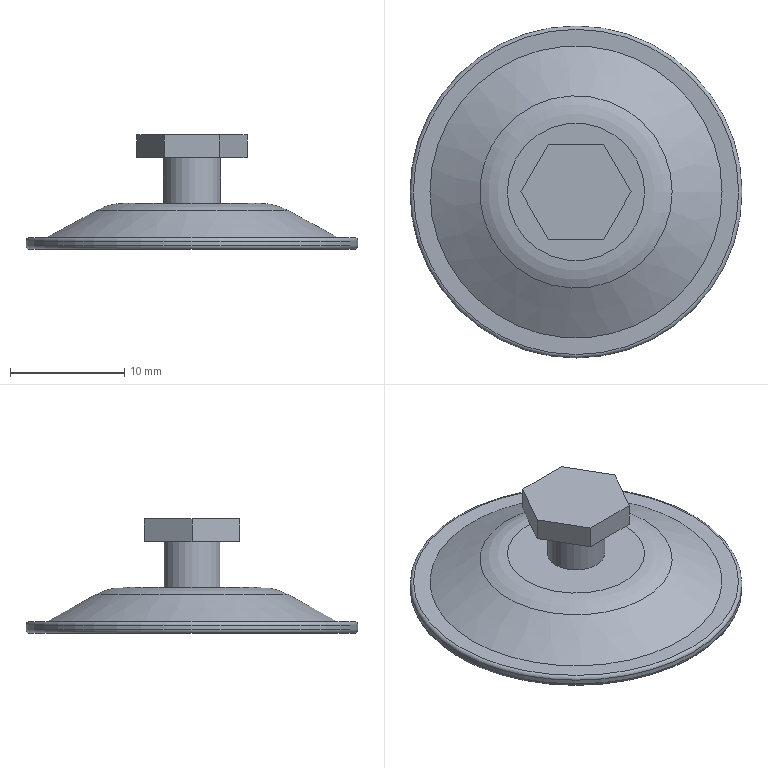Part | STEP file | 1 solid | 22 faces | box 29 x 29 x 10 mm | volume 913.883 mm3 | plane 12 | torus 5 | cylinder 2 | cone 2 | other 1 | commonest cylinder face diameters 5 x1 29 x1
STEP:
#1=CARTESIAN_POINT('',(0.,0.,0.));
#2=DIRECTION('',(0.,0.,1.));
#3=DIRECTION('',(1.,0.,0.));
#4=AXIS2_PLACEMENT_3D('',#1,#2,#3);
#5=CARTESIAN_POINT('',(1541.058,289.48,-116.381));
#6=VERTEX_POINT('',#5);
#7=CARTESIAN_POINT('',(1538.653,285.314,-116.381));
#8=VERTEX_POINT('',#7);
#9=CARTESIAN_POINT('',(1541.058,289.48,-116.381));
#10=DIRECTION('',(-0.5,-0.866,0.));
#11=VECTOR('',#10,1.);
#12=LINE('',#9,#11);
#13=CARTESIAN_POINT('',(1541.058,289.48,-118.381));
#14=DIRECTION('',(-0.866,0.5,0.));
#15=DIRECTION('',(0.5,0.866,0.));
#16=AXIS2_PLACEMENT_3D('',#13,#14,#15);
#17=PLANE('',#16);
#18=CARTESIAN_POINT('',(0.,-2.));
#19=DIRECTION('',(-1.,0.));
#20=VECTOR('',#19,1.);
#21=LINE('',#18,#20);
#22=(GEOMETRIC_REPRESENTATION_CONTEXT(2)PARAMETRIC_REPRESENTATION_CONTEXT()REPRESENTATION_CONTEXT('',''));
#23=DEFINITIONAL_REPRESENTATION('',(#21),#22);
#24=PCURVE('',#17,#23);
#25=CARTESIAN_POINT('',(1536.247,289.48,-116.381));
#26=DIRECTION('',(0.,0.,-1.));
#27=DIRECTION('',(-1.,0.,0.));
#28=AXIS2_PLACEMENT_3D('',#25,#26,#27);
#29=PLANE('',#28);
#30=CARTESIAN_POINT('',(-4.811,0.));
#31=DIRECTION('',(0.5,-0.866));
#32=VECTOR('',#31,1.);
#33=LINE('',#30,#32);
#34=(GEOMETRIC_REPRESENTATION_CONTEXT(2)PARAMETRIC_REPRESENTATION_CONTEXT()REPRESENTATION_CONTEXT('',''));
#35=DEFINITIONAL_REPRESENTATION('',(#33),#34);
#36=PCURVE('',#29,#35);
#37=SURFACE_CURVE('',#12,(#24,#36),.PCURVE_S1.);
#38=EDGE_CURVE('',#6,#8,#37,.T.);
#39=ORIENTED_EDGE('',*,*,#38,.T.);
#40=CARTESIAN_POINT('',(1538.653,285.314,-118.381));
#41=VERTEX_POINT('',#40);
#42=CARTESIAN_POINT('',(1538.653,285.314,-118.381));
#43=DIRECTION('',(0.,0.,1.));
#44=VECTOR('',#43,1.);
#45=LINE('',#42,#44);
#46=CARTESIAN_POINT('',(-4.811,0.));
#47=DIRECTION('',(0.,-1.));
#48=VECTOR('',#47,1.);
#49=LINE('',#46,#48);
#50=(GEOMETRIC_REPRESENTATION_CONTEXT(2)PARAMETRIC_REPRESENTATION_CONTEXT()REPRESENTATION_CONTEXT('',''));
#51=DEFINITIONAL_REPRESENTATION('',(#49),#50);
#52=PCURVE('',#17,#51);
#53=CARTESIAN_POINT('',(1538.653,285.314,-118.381));
#54=DIRECTION('',(0.,1.,0.));
#55=DIRECTION('',(1.,0.,0.));
#56=AXIS2_PLACEMENT_3D('',#53,#54,#55);
#57=PLANE('',#56);
#58=CARTESIAN_POINT('',(0.,0.));
#59=DIRECTION('',(0.,-1.));
#60=VECTOR('',#59,1.);
#61=LINE('',#58,#60);
#62=(GEOMETRIC_REPRESENTATION_CONTEXT(2)PARAMETRIC_REPRESENTATION_CONTEXT()REPRESENTATION_CONTEXT('',''));
#63=DEFINITIONAL_REPRESENTATION('',(#61),#62);
#64=PCURVE('',#57,#63);
#65=SURFACE_CURVE('',#45,(#52,#64),.PCURVE_S1.);
#66=EDGE_CURVE('',#41,#8,#65,.T.);
#67=ORIENTED_EDGE('',*,*,#66,.F.);
#68=CARTESIAN_POINT('',(1541.058,289.48,-118.381));
#69=VERTEX_POINT('',#68);
#70=CARTESIAN_POINT('',(1541.058,289.48,-118.381));
#71=DIRECTION('',(-0.5,-0.866,0.));
#72=VECTOR('',#71,1.);
#73=LINE('',#70,#72);
#74=CARTESIAN_POINT('',(0.,0.));
#75=DIRECTION('',(-1.,0.));
#76=VECTOR('',#75,1.);
#77=LINE('',#74,#76);
#78=(GEOMETRIC_REPRESENTATION_CONTEXT(2)PARAMETRIC_REPRESENTATION_CONTEXT()REPRESENTATION_CONTEXT('',''));
#79=DEFINITIONAL_REPRESENTATION('',(#77),#78);
#80=PCURVE('',#17,#79);
#81=CARTESIAN_POINT('',(1536.247,289.48,-118.381));
#82=DIRECTION('',(0.,0.,-1.));
#83=DIRECTION('',(-1.,0.,0.));
#84=AXIS2_PLACEMENT_3D('',#81,#82,#83);
#85=PLANE('',#84);
#86=CARTESIAN_POINT('',(-4.811,0.));
#87=DIRECTION('',(0.5,-0.866));
#88=VECTOR('',#87,1.);
#89=LINE('',#86,#88);
#90=(GEOMETRIC_REPRESENTATION_CONTEXT(2)PARAMETRIC_REPRESENTATION_CONTEXT()REPRESENTATION_CONTEXT('',''));
#91=DEFINITIONAL_REPRESENTATION('',(#89),#90);
#92=PCURVE('',#85,#91);
#93=SURFACE_CURVE('',#73,(#80,#92),.PCURVE_S1.);
#94=EDGE_CURVE('',#69,#41,#93,.T.);
#95=ORIENTED_EDGE('',*,*,#94,.F.);
#96=CARTESIAN_POINT('',(1541.058,289.48,-118.381));
#97=DIRECTION('',(0.,0.,1.));
#98=VECTOR('',#97,1.);
#99=LINE('',#96,#98);
#100=CARTESIAN_POINT('',(0.,0.));
#101=DIRECTION('',(0.,-1.));
#102=VECTOR('',#101,1.);
#103=LINE('',#100,#102);
#104=(GEOMETRIC_REPRESENTATION_CONTEXT(2)PARAMETRIC_REPRESENTATION_CONTEXT()REPRESENTATION_CONTEXT('',''));
#105=DEFINITIONAL_REPRESENTATION('',(#103),#104);
#106=PCURVE('',#17,#105);
#107=CARTESIAN_POINT('',(1538.653,293.647,-118.381));
#108=DIRECTION('',(-0.866,-0.5,0.));
#109=DIRECTION('',(-0.5,0.866,0.));
#110=AXIS2_PLACEMENT_3D('',#107,#108,#109);
#111=PLANE('',#110);
#112=CARTESIAN_POINT('',(-4.811,0.));
#113=DIRECTION('',(0.,-1.));
#114=VECTOR('',#113,1.);
#115=LINE('',#112,#114);
#116=(GEOMETRIC_REPRESENTATION_CONTEXT(2)PARAMETRIC_REPRESENTATION_CONTEXT()REPRESENTATION_CONTEXT('',''));
#117=DEFINITIONAL_REPRESENTATION('',(#115),#116);
#118=PCURVE('',#111,#117);
#119=SURFACE_CURVE('',#99,(#106,#118),.PCURVE_S1.);
#120=EDGE_CURVE('',#69,#6,#119,.T.);
#121=ORIENTED_EDGE('',*,*,#120,.T.);
#122=EDGE_LOOP('',(#39,#67,#95,#121));
#123=FACE_BOUND('',#122,.T.);
#124=ADVANCED_FACE('',(#123),#17,.F.);
#125=CARTESIAN_POINT('',(1533.842,285.314,-116.381));
#126=VERTEX_POINT('',#125);
#127=CARTESIAN_POINT('',(1538.653,285.314,-116.381));
#128=DIRECTION('',(-1.,0.,0.));
#129=VECTOR('',#128,1.);
#130=LINE('',#127,#129);
#131=CARTESIAN_POINT('',(0.,-2.));
#132=DIRECTION('',(-1.,0.));
#133=VECTOR('',#132,1.);
#134=LINE('',#131,#133);
#135=(GEOMETRIC_REPRESENTATION_CONTEXT(2)PARAMETRIC_REPRESENTATION_CONTEXT()REPRESENTATION_CONTEXT('',''));
#136=DEFINITIONAL_REPRESENTATION('',(#134),#135);
#137=PCURVE('',#57,#136);
#138=CARTESIAN_POINT('',(-2.406,-4.167));
#139=DIRECTION('',(1.,0.));
#140=VECTOR('',#139,1.);
#141=LINE('',#138,#140);
#142=(GEOMETRIC_REPRESENTATION_CONTEXT(2)PARAMETRIC_REPRESENTATION_CONTEXT()REPRESENTATION_CONTEXT('',''));
#143=DEFINITIONAL_REPRESENTATION('',(#141),#142);
#144=PCURVE('',#29,#143);
#145=SURFACE_CURVE('',#130,(#137,#144),.PCURVE_S1.);
#146=EDGE_CURVE('',#8,#126,#145,.T.);
#147=ORIENTED_EDGE('',*,*,#146,.T.);
#148=CARTESIAN_POINT('',(1533.842,285.314,-118.381));
#149=VERTEX_POINT('',#148);
#150=CARTESIAN_POINT('',(1533.842,285.314,-118.381));
#151=DIRECTION('',(0.,0.,1.));
#152=VECTOR('',#151,1.);
#153=LINE('',#150,#152);
#154=CARTESIAN_POINT('',(-4.811,0.));
#155=DIRECTION('',(0.,-1.));
#156=VECTOR('',#155,1.);
#157=LINE('',#154,#156);
#158=(GEOMETRIC_REPRESENTATION_CONTEXT(2)PARAMETRIC_REPRESENTATION_CONTEXT()REPRESENTATION_CONTEXT('',''));
#159=DEFINITIONAL_REPRESENTATION('',(#157),#158);
#160=PCURVE('',#57,#159);
#161=CARTESIAN_POINT('',(1533.842,285.314,-118.381));
#162=DIRECTION('',(0.866,0.5,0.));
#163=DIRECTION('',(0.5,-0.866,0.));
#164=AXIS2_PLACEMENT_3D('',#161,#162,#163);
#165=PLANE('',#164);
#166=CARTESIAN_POINT('',(0.,0.));
#167=DIRECTION('',(0.,-1.));
#168=VECTOR('',#167,1.);
#169=LINE('',#166,#168);
#170=(GEOMETRIC_REPRESENTATION_CONTEXT(2)PARAMETRIC_REPRESENTATION_CONTEXT()REPRESENTATION_CONTEXT('',''));
#171=DEFINITIONAL_REPRESENTATION('',(#169),#170);
#172=PCURVE('',#165,#171);
#173=SURFACE_CURVE('',#153,(#160,#172),.PCURVE_S1.);
#174=EDGE_CURVE('',#149,#126,#173,.T.);
#175=ORIENTED_EDGE('',*,*,#174,.F.);
#176=CARTESIAN_POINT('',(1538.653,285.314,-118.381));
#177=DIRECTION('',(-1.,0.,0.));
#178=VECTOR('',#177,1.);
#179=LINE('',#176,#178);
#180=CARTESIAN_POINT('',(0.,0.));
#181=DIRECTION('',(-1.,0.));
#182=VECTOR('',#181,1.);
#183=LINE('',#180,#182);
#184=(GEOMETRIC_REPRESENTATION_CONTEXT(2)PARAMETRIC_REPRESENTATION_CONTEXT()REPRESENTATION_CONTEXT('',''));
#185=DEFINITIONAL_REPRESENTATION('',(#183),#184);
#186=PCURVE('',#57,#185);
#187=CARTESIAN_POINT('',(-2.406,-4.167));
#188=DIRECTION('',(1.,0.));
#189=VECTOR('',#188,1.);
#190=LINE('',#187,#189);
#191=(GEOMETRIC_REPRESENTATION_CONTEXT(2)PARAMETRIC_REPRESENTATION_CONTEXT()REPRESENTATION_CONTEXT('',''));
#192=DEFINITIONAL_REPRESENTATION('',(#190),#191);
#193=PCURVE('',#85,#192);
#194=SURFACE_CURVE('',#179,(#186,#193),.PCURVE_S1.);
#195=EDGE_CURVE('',#41,#149,#194,.T.);
#196=ORIENTED_EDGE('',*,*,#195,.F.);
#197=ORIENTED_EDGE('',*,*,#66,.T.);
#198=EDGE_LOOP('',(#147,#175,#196,#197));
#199=FACE_BOUND('',#198,.T.);
#200=ADVANCED_FACE('',(#199),#57,.F.);
#201=CARTESIAN_POINT('',(1531.436,289.48,-116.381));
#202=VERTEX_POINT('',#201);
#203=CARTESIAN_POINT('',(1533.842,285.314,-116.381));
#204=DIRECTION('',(-0.5,0.866,0.));
#205=VECTOR('',#204,1.);
#206=LINE('',#203,#205);
#207=CARTESIAN_POINT('',(0.,-2.));
#208=DIRECTION('',(-1.,0.));
#209=VECTOR('',#208,1.);
#210=LINE('',#207,#209);
#211=(GEOMETRIC_REPRESENTATION_CONTEXT(2)PARAMETRIC_REPRESENTATION_CONTEXT()REPRESENTATION_CONTEXT('',''));
#212=DEFINITIONAL_REPRESENTATION('',(#210),#211);
#213=PCURVE('',#165,#212);
#214=CARTESIAN_POINT('',(2.406,-4.167));
#215=DIRECTION('',(0.5,0.866));
#216=VECTOR('',#215,1.);
#217=LINE('',#214,#216);
#218=(GEOMETRIC_REPRESENTATION_CONTEXT(2)PARAMETRIC_REPRESENTATION_CONTEXT()REPRESENTATION_CONTEXT('',''));
#219=DEFINITIONAL_REPRESENTATION('',(#217),#218);
#220=PCURVE('',#29,#219);
#221=SURFACE_CURVE('',#206,(#213,#220),.PCURVE_S1.);
#222=EDGE_CURVE('',#126,#202,#221,.T.);
#223=ORIENTED_EDGE('',*,*,#222,.T.);
#224=CARTESIAN_POINT('',(1531.436,289.48,-118.381));
#225=VERTEX_POINT('',#224);
#226=CARTESIAN_POINT('',(1531.436,289.48,-118.381));
#227=DIRECTION('',(0.,0.,1.));
#228=VECTOR('',#227,1.);
#229=LINE('',#226,#228);
#230=CARTESIAN_POINT('',(-4.811,0.));
#231=DIRECTION('',(0.,-1.));
#232=VECTOR('',#231,1.);
#233=LINE('',#230,#232);
#234=(GEOMETRIC_REPRESENTATION_CONTEXT(2)PARAMETRIC_REPRESENTATION_CONTEXT()REPRESENTATION_CONTEXT('',''));
#235=DEFINITIONAL_REPRESENTATION('',(#233),#234);
#236=PCURVE('',#165,#235);
#237=CARTESIAN_POINT('',(1531.436,289.48,-118.381));
#238=DIRECTION('',(0.866,-0.5,0.));
#239=DIRECTION('',(-0.5,-0.866,0.));
#240=AXIS2_PLACEMENT_3D('',#237,#238,#239);
#241=PLANE('',#240);
#242=CARTESIAN_POINT('',(0.,0.));
#243=DIRECTION('',(0.,-1.));
#244=VECTOR('',#243,1.);
#245=LINE('',#242,#244);
#246=(GEOMETRIC_REPRESENTATION_CONTEXT(2)PARAMETRIC_REPRESENTATION_CONTEXT()REPRESENTATION_CONTEXT('',''));
#247=DEFINITIONAL_REPRESENTATION('',(#245),#246);
#248=PCURVE('',#241,#247);
#249=SURFACE_CURVE('',#229,(#236,#248),.PCURVE_S1.);
#250=EDGE_CURVE('',#225,#202,#249,.T.);
#251=ORIENTED_EDGE('',*,*,#250,.F.);
#252=CARTESIAN_POINT('',(1533.842,285.314,-118.381));
#253=DIRECTION('',(-0.5,0.866,0.));
#254=VECTOR('',#253,1.);
#255=LINE('',#252,#254);
#256=CARTESIAN_POINT('',(0.,0.));
#257=DIRECTION('',(-1.,0.));
#258=VECTOR('',#257,1.);
#259=LINE('',#256,#258);
#260=(GEOMETRIC_REPRESENTATION_CONTEXT(2)PARAMETRIC_REPRESENTATION_CONTEXT()REPRESENTATION_CONTEXT('',''));
#261=DEFINITIONAL_REPRESENTATION('',(#259),#260);
#262=PCURVE('',#165,#261);
#263=CARTESIAN_POINT('',(2.406,-4.167));
#264=DIRECTION('',(0.5,0.866));
#265=VECTOR('',#264,1.);
#266=LINE('',#263,#265);
#267=(GEOMETRIC_REPRESENTATION_CONTEXT(2)PARAMETRIC_REPRESENTATION_CONTEXT()REPRESENTATION_CONTEXT('',''));
#268=DEFINITIONAL_REPRESENTATION('',(#266),#267);
#269=PCURVE('',#85,#268);
#270=SURFACE_CURVE('',#255,(#262,#269),.PCURVE_S1.);
#271=EDGE_CURVE('',#149,#225,#270,.T.);
#272=ORIENTED_EDGE('',*,*,#271,.F.);
#273=ORIENTED_EDGE('',*,*,#174,.T.);
#274=EDGE_LOOP('',(#223,#251,#272,#273));
#275=FACE_BOUND('',#274,.T.);
#276=ADVANCED_FACE('',(#275),#165,.F.);
#277=CARTESIAN_POINT('',(1533.842,293.647,-116.381));
#278=VERTEX_POINT('',#277);
#279=CARTESIAN_POINT('',(1531.436,289.48,-116.381));
#280=DIRECTION('',(0.5,0.866,0.));
#281=VECTOR('',#280,1.);
#282=LINE('',#279,#281);
#283=CARTESIAN_POINT('',(0.,-2.));
#284=DIRECTION('',(-1.,0.));
#285=VECTOR('',#284,1.);
#286=LINE('',#283,#285);
#287=(GEOMETRIC_REPRESENTATION_CONTEXT(2)PARAMETRIC_REPRESENTATION_CONTEXT()REPRESENTATION_CONTEXT('',''));
#288=DEFINITIONAL_REPRESENTATION('',(#286),#287);
#289=PCURVE('',#241,#288);
#290=CARTESIAN_POINT('',(4.811,0.));
#291=DIRECTION('',(-0.5,0.866));
#292=VECTOR('',#291,1.);
#293=LINE('',#290,#292);
#294=(GEOMETRIC_REPRESENTATION_CONTEXT(2)PARAMETRIC_REPRESENTATION_CONTEXT()REPRESENTATION_CONTEXT('',''));
#295=DEFINITIONAL_REPRESENTATION('',(#293),#294);
#296=PCURVE('',#29,#295);
#297=SURFACE_CURVE('',#282,(#289,#296),.PCURVE_S1.);
#298=EDGE_CURVE('',#202,#278,#297,.T.);
#299=ORIENTED_EDGE('',*,*,#298,.T.);
#300=CARTESIAN_POINT('',(1533.842,293.647,-118.381));
#301=VERTEX_POINT('',#300);
#302=CARTESIAN_POINT('',(1533.842,293.647,-118.381));
#303=DIRECTION('',(0.,0.,1.));
#304=VECTOR('',#303,1.);
#305=LINE('',#302,#304);
#306=CARTESIAN_POINT('',(-4.811,0.));
#307=DIRECTION('',(0.,-1.));
#308=VECTOR('',#307,1.);
#309=LINE('',#306,#308);
#310=(GEOMETRIC_REPRESENTATION_CONTEXT(2)PARAMETRIC_REPRESENTATION_CONTEXT()REPRESENTATION_CONTEXT('',''));
#311=DEFINITIONAL_REPRESENTATION('',(#309),#310);
#312=PCURVE('',#241,#311);
#313=CARTESIAN_POINT('',(1533.842,293.647,-118.381));
#314=DIRECTION('',(0.,-1.,0.));
#315=DIRECTION('',(-1.,0.,0.));
#316=AXIS2_PLACEMENT_3D('',#313,#314,#315);
#317=PLANE('',#316);
#318=CARTESIAN_POINT('',(0.,0.));
#319=DIRECTION('',(0.,-1.));
#320=VECTOR('',#319,1.);
#321=LINE('',#318,#320);
#322=(GEOMETRIC_REPRESENTATION_CONTEXT(2)PARAMETRIC_REPRESENTATION_CONTEXT()REPRESENTATION_CONTEXT('',''));
#323=DEFINITIONAL_REPRESENTATION('',(#321),#322);
#324=PCURVE('',#317,#323);
#325=SURFACE_CURVE('',#305,(#312,#324),.PCURVE_S1.);
#326=EDGE_CURVE('',#301,#278,#325,.T.);
#327=ORIENTED_EDGE('',*,*,#326,.F.);
#328=CARTESIAN_POINT('',(1531.436,289.48,-118.381));
#329=DIRECTION('',(0.5,0.866,0.));
#330=VECTOR('',#329,1.);
#331=LINE('',#328,#330);
#332=CARTESIAN_POINT('',(0.,0.));
#333=DIRECTION('',(-1.,0.));
#334=VECTOR('',#333,1.);
#335=LINE('',#332,#334);
#336=(GEOMETRIC_REPRESENTATION_CONTEXT(2)PARAMETRIC_REPRESENTATION_CONTEXT()REPRESENTATION_CONTEXT('',''));
#337=DEFINITIONAL_REPRESENTATION('',(#335),#336);
#338=PCURVE('',#241,#337);
#339=CARTESIAN_POINT('',(4.811,0.));
#340=DIRECTION('',(-0.5,0.866));
#341=VECTOR('',#340,1.);
#342=LINE('',#339,#341);
#343=(GEOMETRIC_REPRESENTATION_CONTEXT(2)PARAMETRIC_REPRESENTATION_CONTEXT()REPRESENTATION_CONTEXT('',''));
#344=DEFINITIONAL_REPRESENTATION('',(#342),#343);
#345=PCURVE('',#85,#344);
#346=SURFACE_CURVE('',#331,(#338,#345),.PCURVE_S1.);
#347=EDGE_CURVE('',#225,#301,#346,.T.);
#348=ORIENTED_EDGE('',*,*,#347,.F.);
#349=ORIENTED_EDGE('',*,*,#250,.T.);
#350=EDGE_LOOP('',(#299,#327,#348,#349));
#351=FACE_BOUND('',#350,.T.);
#352=ADVANCED_FACE('',(#351),#241,.F.);
#353=CARTESIAN_POINT('',(1538.653,293.647,-116.381));
#354=VERTEX_POINT('',#353);
#355=CARTESIAN_POINT('',(1533.842,293.647,-116.381));
#356=DIRECTION('',(1.,0.,0.));
#357=VECTOR('',#356,1.);
#358=LINE('',#355,#357);
#359=CARTESIAN_POINT('',(0.,-2.));
#360=DIRECTION('',(-1.,0.));
#361=VECTOR('',#360,1.);
#362=LINE('',#359,#361);
#363=(GEOMETRIC_REPRESENTATION_CONTEXT(2)PARAMETRIC_REPRESENTATION_CONTEXT()REPRESENTATION_CONTEXT('',''));
#364=DEFINITIONAL_REPRESENTATION('',(#362),#363);
#365=PCURVE('',#317,#364);
#366=CARTESIAN_POINT('',(2.406,4.167));
#367=DIRECTION('',(-1.,0.));
#368=VECTOR('',#367,1.);
#369=LINE('',#366,#368);
#370=(GEOMETRIC_REPRESENTATION_CONTEXT(2)PARAMETRIC_REPRESENTATION_CONTEXT()REPRESENTATION_CONTEXT('',''));
#371=DEFINITIONAL_REPRESENTATION('',(#369),#370);
#372=PCURVE('',#29,#371);
#373=SURFACE_CURVE('',#358,(#365,#372),.PCURVE_S1.);
#374=EDGE_CURVE('',#278,#354,#373,.T.);
#375=ORIENTED_EDGE('',*,*,#374,.T.);
#376=CARTESIAN_POINT('',(1538.653,293.647,-118.381));
#377=VERTEX_POINT('',#376);
#378=CARTESIAN_POINT('',(1538.653,293.647,-118.381));
#379=DIRECTION('',(0.,0.,1.));
#380=VECTOR('',#379,1.);
#381=LINE('',#378,#380);
#382=CARTESIAN_POINT('',(-4.811,0.));
#383=DIRECTION('',(0.,-1.));
#384=VECTOR('',#383,1.);
#385=LINE('',#382,#384);
#386=(GEOMETRIC_REPRESENTATION_CONTEXT(2)PARAMETRIC_REPRESENTATION_CONTEXT()REPRESENTATION_CONTEXT('',''));
#387=DEFINITIONAL_REPRESENTATION('',(#385),#386);
#388=PCURVE('',#317,#387);
#389=CARTESIAN_POINT('',(0.,0.));
#390=DIRECTION('',(0.,-1.));
#391=VECTOR('',#390,1.);
#392=LINE('',#389,#391);
#393=(GEOMETRIC_REPRESENTATION_CONTEXT(2)PARAMETRIC_REPRESENTATION_CONTEXT()REPRESENTATION_CONTEXT('',''));
#394=DEFINITIONAL_REPRESENTATION('',(#392),#393);
#395=PCURVE('',#111,#394);
#396=SURFACE_CURVE('',#381,(#388,#395),.PCURVE_S1.);
#397=EDGE_CURVE('',#377,#354,#396,.T.);
#398=ORIENTED_EDGE('',*,*,#397,.F.);
#399=CARTESIAN_POINT('',(1533.842,293.647,-118.381));
#400=DIRECTION('',(1.,0.,0.));
#401=VECTOR('',#400,1.);
#402=LINE('',#399,#401);
#403=CARTESIAN_POINT('',(0.,0.));
#404=DIRECTION('',(-1.,0.));
#405=VECTOR('',#404,1.);
#406=LINE('',#403,#405);
#407=(GEOMETRIC_REPRESENTATION_CONTEXT(2)PARAMETRIC_REPRESENTATION_CONTEXT()REPRESENTATION_CONTEXT('',''));
#408=DEFINITIONAL_REPRESENTATION('',(#406),#407);
#409=PCURVE('',#317,#408);
#410=CARTESIAN_POINT('',(2.406,4.167));
#411=DIRECTION('',(-1.,0.));
#412=VECTOR('',#411,1.);
#413=LINE('',#410,#412);
#414=(GEOMETRIC_REPRESENTATION_CONTEXT(2)PARAMETRIC_REPRESENTATION_CONTEXT()REPRESENTATION_CONTEXT('',''));
#415=DEFINITIONAL_REPRESENTATION('',(#413),#414);
#416=PCURVE('',#85,#415);
#417=SURFACE_CURVE('',#402,(#409,#416),.PCURVE_S1.);
#418=EDGE_CURVE('',#301,#377,#417,.T.);
#419=ORIENTED_EDGE('',*,*,#418,.F.);
#420=ORIENTED_EDGE('',*,*,#326,.T.);
#421=EDGE_LOOP('',(#375,#398,#419,#420));
#422=FACE_BOUND('',#421,.T.);
#423=ADVANCED_FACE('',(#422),#317,.F.);
#424=CARTESIAN_POINT('',(1538.653,293.647,-116.381));
#425=DIRECTION('',(0.5,-0.866,0.));
#426=VECTOR('',#425,1.);
#427=LINE('',#424,#426);
#428=CARTESIAN_POINT('',(0.,-2.));
#429=DIRECTION('',(-1.,0.));
#430=VECTOR('',#429,1.);
#431=LINE('',#428,#430);
#432=(GEOMETRIC_REPRESENTATION_CONTEXT(2)PARAMETRIC_REPRESENTATION_CONTEXT()REPRESENTATION_CONTEXT('',''));
#433=DEFINITIONAL_REPRESENTATION('',(#431),#432);
#434=PCURVE('',#111,#433);
#435=CARTESIAN_POINT('',(-2.406,4.167));
#436=DIRECTION('',(-0.5,-0.866));
#437=VECTOR('',#436,1.);
#438=LINE('',#435,#437);
#439=(GEOMETRIC_REPRESENTATION_CONTEXT(2)PARAMETRIC_REPRESENTATION_CONTEXT()REPRESENTATION_CONTEXT('',''));
#440=DEFINITIONAL_REPRESENTATION('',(#438),#439);
#441=PCURVE('',#29,#440);
#442=SURFACE_CURVE('',#427,(#434,#441),.PCURVE_S1.);
#443=EDGE_CURVE('',#354,#6,#442,.T.);
#444=ORIENTED_EDGE('',*,*,#443,.T.);
#445=ORIENTED_EDGE('',*,*,#120,.F.);
#446=CARTESIAN_POINT('',(1538.653,293.647,-118.381));
#447=DIRECTION('',(0.5,-0.866,0.));
#448=VECTOR('',#447,1.);
#449=LINE('',#446,#448);
#450=CARTESIAN_POINT('',(0.,0.));
#451=DIRECTION('',(-1.,0.));
#452=VECTOR('',#451,1.);
#453=LINE('',#450,#452);
#454=(GEOMETRIC_REPRESENTATION_CONTEXT(2)PARAMETRIC_REPRESENTATION_CONTEXT()REPRESENTATION_CONTEXT('',''));
#455=DEFINITIONAL_REPRESENTATION('',(#453),#454);
#456=PCURVE('',#111,#455);
#457=CARTESIAN_POINT('',(-2.406,4.167));
#458=DIRECTION('',(-0.5,-0.866));
#459=VECTOR('',#458,1.);
#460=LINE('',#457,#459);
#461=(GEOMETRIC_REPRESENTATION_CONTEXT(2)PARAMETRIC_REPRESENTATION_CONTEXT()REPRESENTATION_CONTEXT('',''));
#462=DEFINITIONAL_REPRESENTATION('',(#460),#461);
#463=PCURVE('',#85,#462);
#464=SURFACE_CURVE('',#449,(#456,#463),.PCURVE_S1.);
#465=EDGE_CURVE('',#377,#69,#464,.T.);
#466=ORIENTED_EDGE('',*,*,#465,.F.);
#467=ORIENTED_EDGE('',*,*,#397,.T.);
#468=EDGE_LOOP('',(#444,#445,#466,#467));
#469=FACE_BOUND('',#468,.T.);
#470=ADVANCED_FACE('',(#469),#111,.F.);
#471=CARTESIAN_POINT('',(1533.747,289.48,-118.381));
#472=VERTEX_POINT('',#471);
#473=CARTESIAN_POINT('',(1538.747,289.48,-118.381));
#474=VERTEX_POINT('',#473);
#475=CARTESIAN_POINT('',(1536.247,289.48,-118.381));
#476=DIRECTION('',(0.,0.,-1.));
#477=DIRECTION('',(-1.,0.,0.));
#478=AXIS2_PLACEMENT_3D('',#475,#476,#477);
#479=CIRCLE('',#478,2.5);
#480=CARTESIAN_POINT('',(0.,0.));
#481=DIRECTION('',(1.,0.));
#482=AXIS2_PLACEMENT_2D('',#480,#481);
#483=CIRCLE('',#482,2.5);
#484=(GEOMETRIC_REPRESENTATION_CONTEXT(2)PARAMETRIC_REPRESENTATION_CONTEXT()REPRESENTATION_CONTEXT('',''));
#485=DEFINITIONAL_REPRESENTATION('',(#483),#484);
#486=PCURVE('',#85,#485);
#487=CARTESIAN_POINT('',(1536.247,289.48,-116.381));
#488=DIRECTION('',(0.,0.,1.));
#489=DIRECTION('',(1.,0.,0.));
#490=AXIS2_PLACEMENT_3D('',#487,#488,#489);
#491=CYLINDRICAL_SURFACE('',#490,2.5);
#492=CARTESIAN_POINT('',(3.142,-2.));
#493=DIRECTION('',(-1.,0.));
#494=VECTOR('',#493,1.);
#495=LINE('',#492,#494);
#496=(GEOMETRIC_REPRESENTATION_CONTEXT(2)PARAMETRIC_REPRESENTATION_CONTEXT()REPRESENTATION_CONTEXT('',''));
#497=DEFINITIONAL_REPRESENTATION('',(#495),#496);
#498=PCURVE('',#491,#497);
#499=SURFACE_CURVE('',#479,(#486,#498),.PCURVE_S1.);
#500=EDGE_CURVE('',#472,#474,#499,.T.);
#501=ORIENTED_EDGE('',*,*,#500,.F.);
#502=CARTESIAN_POINT('',(1536.247,289.48,-118.381));
#503=DIRECTION('',(0.,0.,-1.));
#504=DIRECTION('',(-1.,0.,0.));
#505=AXIS2_PLACEMENT_3D('',#502,#503,#504);
#506=CIRCLE('',#505,2.5);
#507=CARTESIAN_POINT('',(0.,0.));
#508=DIRECTION('',(1.,0.));
#509=AXIS2_PLACEMENT_2D('',#507,#508);
#510=CIRCLE('',#509,2.5);
#511=(GEOMETRIC_REPRESENTATION_CONTEXT(2)PARAMETRIC_REPRESENTATION_CONTEXT()REPRESENTATION_CONTEXT('',''));
#512=DEFINITIONAL_REPRESENTATION('',(#510),#511);
#513=PCURVE('',#85,#512);
#514=CARTESIAN_POINT('',(9.425,-2.));
#515=DIRECTION('',(-1.,0.));
#516=VECTOR('',#515,1.);
#517=LINE('',#514,#516);
#518=(GEOMETRIC_REPRESENTATION_CONTEXT(2)PARAMETRIC_REPRESENTATION_CONTEXT()REPRESENTATION_CONTEXT('',''));
#519=DEFINITIONAL_REPRESENTATION('',(#517),#518);
#520=PCURVE('',#491,#519);
#521=SURFACE_CURVE('',#506,(#513,#520),.PCURVE_S1.);
#522=EDGE_CURVE('',#474,#472,#521,.T.);
#523=ORIENTED_EDGE('',*,*,#522,.F.);
#524=EDGE_LOOP('',(#501,#523));
#525=FACE_BOUND('',#524,.T.);
#526=ORIENTED_EDGE('',*,*,#94,.T.);
#527=ORIENTED_EDGE('',*,*,#195,.T.);
#528=ORIENTED_EDGE('',*,*,#271,.T.);
#529=ORIENTED_EDGE('',*,*,#347,.T.);
#530=ORIENTED_EDGE('',*,*,#418,.T.);
#531=ORIENTED_EDGE('',*,*,#465,.T.);
#532=EDGE_LOOP('',(#526,#527,#528,#529,#530,#531));
#533=FACE_BOUND('',#532,.T.);
#534=ADVANCED_FACE('',(#525,#533),#85,.T.);
#535=ORIENTED_EDGE('',*,*,#500,.T.);
#536=CARTESIAN_POINT('',(1538.747,289.48,-122.381));
#537=VERTEX_POINT('',#536);
#538=CARTESIAN_POINT('',(1538.747,289.48,-122.381));
#539=CARTESIAN_POINT('',(1538.747,289.48,-118.381));
#540=B_SPLINE_CURVE_WITH_KNOTS('',1,(#538,#539),.UNSPECIFIED.,.F.,.F.,(2,2),(-6.,-2.),.PIECEWISE_BEZIER_KNOTS.);
#541=CARTESIAN_POINT('',(0.,0.));
#542=DIRECTION('',(0.,1.));
#543=VECTOR('',#542,1.);
#544=LINE('',#541,#543);
#545=(GEOMETRIC_REPRESENTATION_CONTEXT(2)PARAMETRIC_REPRESENTATION_CONTEXT()REPRESENTATION_CONTEXT('',''));
#546=DEFINITIONAL_REPRESENTATION('',(#544),#545);
#547=PCURVE('',#491,#546);
#548=CARTESIAN_POINT('',(6.283,0.));
#549=DIRECTION('',(0.,1.));
#550=VECTOR('',#549,1.);
#551=LINE('',#548,#550);
#552=(GEOMETRIC_REPRESENTATION_CONTEXT(2)PARAMETRIC_REPRESENTATION_CONTEXT()REPRESENTATION_CONTEXT('',''));
#553=DEFINITIONAL_REPRESENTATION('',(#551),#552);
#554=PCURVE('',#491,#553);
#555=SEAM_CURVE('',#540,(#547,#554),.PCURVE_S1.);
#556=EDGE_CURVE('',#537,#474,#555,.T.);
#557=ORIENTED_EDGE('',*,*,#556,.F.);
#558=CARTESIAN_POINT('',(1536.247,289.48,-122.381));
#559=DIRECTION('',(0.,0.,1.));
#560=DIRECTION('',(1.,0.,0.));
#561=AXIS2_PLACEMENT_3D('',#558,#559,#560);
#562=CIRCLE('',#561,2.5);
#563=CARTESIAN_POINT('',(0.,-6.));
#564=DIRECTION('',(1.,0.));
#565=VECTOR('',#564,1.);
#566=LINE('',#563,#565);
#567=(GEOMETRIC_REPRESENTATION_CONTEXT(2)PARAMETRIC_REPRESENTATION_CONTEXT()REPRESENTATION_CONTEXT('',''));
#568=DEFINITIONAL_REPRESENTATION('',(#566),#567);
#569=PCURVE('',#491,#568);
#570=CARTESIAN_POINT('',(1533.747,289.48,-122.381));
#571=DIRECTION('',(0.,0.,1.));
#572=DIRECTION('',(1.,0.,0.));
#573=AXIS2_PLACEMENT_3D('',#570,#571,#572);
#574=PLANE('',#573);
#575=CARTESIAN_POINT('',(2.5,0.));
#576=DIRECTION('',(1.,0.));
#577=AXIS2_PLACEMENT_2D('',#575,#576);
#578=CIRCLE('',#577,2.5);
#579=(GEOMETRIC_REPRESENTATION_CONTEXT(2)PARAMETRIC_REPRESENTATION_CONTEXT()REPRESENTATION_CONTEXT('',''));
#580=DEFINITIONAL_REPRESENTATION('',(#578),#579);
#581=PCURVE('',#574,#580);
#582=SURFACE_CURVE('',#562,(#569,#581),.PCURVE_S1.);
#583=EDGE_CURVE('',#537,#537,#582,.T.);
#584=ORIENTED_EDGE('',*,*,#583,.T.);
#585=ORIENTED_EDGE('',*,*,#556,.T.);
#586=ORIENTED_EDGE('',*,*,#522,.T.);
#587=EDGE_LOOP('',(#535,#557,#584,#585,#586));
#588=FACE_BOUND('',#587,.T.);
#589=ADVANCED_FACE('',(#588),#491,.T.);
#590=CARTESIAN_POINT('',(1542.247,289.48,-122.381));
#591=VERTEX_POINT('',#590);
#592=CARTESIAN_POINT('',(1536.247,289.48,-122.381));
#593=DIRECTION('',(0.,0.,1.));
#594=DIRECTION('',(1.,0.,0.));
#595=AXIS2_PLACEMENT_3D('',#592,#593,#594);
#596=CIRCLE('',#595,6.);
#597=CARTESIAN_POINT('',(2.5,0.));
#598=DIRECTION('',(1.,0.));
#599=AXIS2_PLACEMENT_2D('',#597,#598);
#600=CIRCLE('',#599,6.);
#601=(GEOMETRIC_REPRESENTATION_CONTEXT(2)PARAMETRIC_REPRESENTATION_CONTEXT()REPRESENTATION_CONTEXT('',''));
#602=DEFINITIONAL_REPRESENTATION('',(#600),#601);
#603=PCURVE('',#574,#602);
#604=CARTESIAN_POINT('',(1536.247,289.48,-127.381));
#605=DIRECTION('',(0.,0.,1.));
#606=DIRECTION('',(1.,0.,0.));
#607=AXIS2_PLACEMENT_3D('',#604,#605,#606);
#608=TOROIDAL_SURFACE('',#607,6.,5.);
#609=CARTESIAN_POINT('',(0.,7.854));
#610=DIRECTION('',(1.,0.));
#611=VECTOR('',#610,1.);
#612=LINE('',#609,#611);
#613=(GEOMETRIC_REPRESENTATION_CONTEXT(2)PARAMETRIC_REPRESENTATION_CONTEXT()REPRESENTATION_CONTEXT('',''));
#614=DEFINITIONAL_REPRESENTATION('',(#612),#613);
#615=PCURVE('',#608,#614);
#616=SURFACE_CURVE('',#596,(#603,#615),.PCURVE_S1.);
#617=EDGE_CURVE('',#591,#591,#616,.T.);
#618=ORIENTED_EDGE('',*,*,#617,.T.);
#619=EDGE_LOOP('',(#618));
#620=FACE_BOUND('',#619,.T.);
#621=ORIENTED_EDGE('',*,*,#583,.F.);
#622=EDGE_LOOP('',(#621));
#623=FACE_BOUND('',#622,.T.);
#624=ADVANCED_FACE('',(#620,#623),#574,.T.);
#625=CARTESIAN_POINT('',(1544.649,289.48,-122.996));
#626=VERTEX_POINT('',#625);
#627=CARTESIAN_POINT('',(1536.247,289.48,-122.996));
#628=DIRECTION('',(0.,0.,1.));
#629=DIRECTION('',(1.,0.,0.));
#630=AXIS2_PLACEMENT_3D('',#627,#628,#629);
#631=CIRCLE('',#630,8.402);
#632=CARTESIAN_POINT('',(0.,7.353));
#633=DIRECTION('',(1.,0.));
#634=VECTOR('',#633,1.);
#635=LINE('',#632,#634);
#636=(GEOMETRIC_REPRESENTATION_CONTEXT(2)PARAMETRIC_REPRESENTATION_CONTEXT()REPRESENTATION_CONTEXT('',''));
#637=DEFINITIONAL_REPRESENTATION('',(#635),#636);
#638=PCURVE('',#608,#637);
#639=CARTESIAN_POINT('',(1536.247,289.48,-122.996));
#640=DIRECTION('',(0.,0.,-1.));
#641=DIRECTION('',(-1.,0.,0.));
#642=AXIS2_PLACEMENT_3D('',#639,#640,#641);
#643=CONICAL_SURFACE('',#642,8.402,1.07);
#644=CARTESIAN_POINT('',(9.425,0.));
#645=DIRECTION('',(-1.,0.));
#646=VECTOR('',#645,1.);
#647=LINE('',#644,#646);
#648=(GEOMETRIC_REPRESENTATION_CONTEXT(2)PARAMETRIC_REPRESENTATION_CONTEXT()REPRESENTATION_CONTEXT('',''));
#649=DEFINITIONAL_REPRESENTATION('',(#647),#648);
#650=PCURVE('',#643,#649);
#651=SURFACE_CURVE('',#631,(#638,#650),.PCURVE_S1.);
#652=EDGE_CURVE('',#626,#626,#651,.T.);
#653=ORIENTED_EDGE('',*,*,#652,.T.);
#654=CARTESIAN_POINT('',(1544.649,289.48,-122.996));
#655=CARTESIAN_POINT('',(1544.282,289.48,-122.795));
#656=CARTESIAN_POINT('',(1543.896,289.48,-122.631));
#657=CARTESIAN_POINT('',(1543.495,289.48,-122.507));
#658=CARTESIAN_POINT('',(1543.083,289.48,-122.423));
#659=CARTESIAN_POINT('',(1542.666,289.48,-122.381));
#660=CARTESIAN_POINT('',(1542.247,289.48,-122.381));
#661=(BOUNDED_CURVE()B_SPLINE_CURVE(6,(#654,#655,#656,#657,#658,#659,#660),.UNSPECIFIED.,.F.,.F.)B_SPLINE_CURVE_WITH_KNOTS((7,7),(1.07,1.571),.PIECEWISE_BEZIER_KNOTS.)CURVE()GEOMETRIC_REPRESENTATION_ITEM()RATIONAL_B_SPLINE_CURVE((1.003,1.001,0.9998,0.9994,0.9998,1.001,1.003))REPRESENTATION_ITEM(''));
#662=CARTESIAN_POINT('',(6.283,6.283));
#663=DIRECTION('',(0.,1.));
#664=VECTOR('',#663,1.);
#665=LINE('',#662,#664);
#666=(GEOMETRIC_REPRESENTATION_CONTEXT(2)PARAMETRIC_REPRESENTATION_CONTEXT()REPRESENTATION_CONTEXT('',''));
#667=DEFINITIONAL_REPRESENTATION('',(#665),#666);
#668=PCURVE('',#608,#667);
#669=CARTESIAN_POINT('',(0.,6.283));
#670=DIRECTION('',(0.,1.));
#671=VECTOR('',#670,1.);
#672=LINE('',#669,#671);
#673=(GEOMETRIC_REPRESENTATION_CONTEXT(2)PARAMETRIC_REPRESENTATION_CONTEXT()REPRESENTATION_CONTEXT('',''));
#674=DEFINITIONAL_REPRESENTATION('',(#672),#673);
#675=PCURVE('',#608,#674);
#676=SEAM_CURVE('',#661,(#668,#675),.PCURVE_S1.);
#677=EDGE_CURVE('',#626,#591,#676,.T.);
#678=ORIENTED_EDGE('',*,*,#677,.T.);
#679=ORIENTED_EDGE('',*,*,#617,.F.);
#680=ORIENTED_EDGE('',*,*,#677,.F.);
#681=EDGE_LOOP('',(#653,#678,#679,#680));
#682=FACE_BOUND('',#681,.T.);
#683=ADVANCED_FACE('',(#682),#608,.T.);
#684=CARTESIAN_POINT('',(1549.003,289.48,-125.381));
#685=VERTEX_POINT('',#684);
#686=CARTESIAN_POINT('',(1536.247,289.48,-125.381));
#687=DIRECTION('',(0.,0.,1.));
#688=DIRECTION('',(1.,0.,0.));
#689=AXIS2_PLACEMENT_3D('',#686,#687,#688);
#690=CIRCLE('',#689,12.756);
#691=CARTESIAN_POINT('',(9.425,2.385));
#692=DIRECTION('',(-1.,0.));
#693=VECTOR('',#692,1.);
#694=LINE('',#691,#693);
#695=(GEOMETRIC_REPRESENTATION_CONTEXT(2)PARAMETRIC_REPRESENTATION_CONTEXT()REPRESENTATION_CONTEXT('',''));
#696=DEFINITIONAL_REPRESENTATION('',(#694),#695);
#697=PCURVE('',#643,#696);
#698=CARTESIAN_POINT('',(1523.491,289.48,-125.381));
#699=DIRECTION('',(0.,0.,1.));
#700=DIRECTION('',(1.,0.,0.));
#701=AXIS2_PLACEMENT_3D('',#698,#699,#700);
#702=PLANE('',#701);
#703=CARTESIAN_POINT('',(12.756,0.));
#704=DIRECTION('',(1.,0.));
#705=AXIS2_PLACEMENT_2D('',#703,#704);
#706=CIRCLE('',#705,12.756);
#707=(GEOMETRIC_REPRESENTATION_CONTEXT(2)PARAMETRIC_REPRESENTATION_CONTEXT()REPRESENTATION_CONTEXT('',''));
#708=DEFINITIONAL_REPRESENTATION('',(#706),#707);
#709=PCURVE('',#702,#708);
#710=SURFACE_CURVE('',#690,(#697,#709),.PCURVE_S1.);
#711=EDGE_CURVE('',#685,#685,#710,.T.);
#712=ORIENTED_EDGE('',*,*,#711,.T.);
#713=CARTESIAN_POINT('',(1544.649,289.48,-122.996));
#714=CARTESIAN_POINT('',(1549.003,289.48,-125.381));
#715=B_SPLINE_CURVE_WITH_KNOTS('',1,(#713,#714),.UNSPECIFIED.,.F.,.F.,(2,2),(0.,4.964),.PIECEWISE_BEZIER_KNOTS.);
#716=CARTESIAN_POINT('',(3.142,0.));
#717=DIRECTION('',(0.,1.));
#718=VECTOR('',#717,1.);
#719=LINE('',#716,#718);
#720=(GEOMETRIC_REPRESENTATION_CONTEXT(2)PARAMETRIC_REPRESENTATION_CONTEXT()REPRESENTATION_CONTEXT('',''));
#721=DEFINITIONAL_REPRESENTATION('',(#719),#720);
#722=PCURVE('',#643,#721);
#723=CARTESIAN_POINT('',(9.425,0.));
#724=DIRECTION('',(0.,1.));
#725=VECTOR('',#724,1.);
#726=LINE('',#723,#725);
#727=(GEOMETRIC_REPRESENTATION_CONTEXT(2)PARAMETRIC_REPRESENTATION_CONTEXT()REPRESENTATION_CONTEXT('',''));
#728=DEFINITIONAL_REPRESENTATION('',(#726),#727);
#729=PCURVE('',#643,#728);
#730=SEAM_CURVE('',#715,(#722,#729),.PCURVE_S1.);
#731=EDGE_CURVE('',#626,#685,#730,.T.);
#732=ORIENTED_EDGE('',*,*,#731,.F.);
#733=ORIENTED_EDGE('',*,*,#652,.F.);
#734=ORIENTED_EDGE('',*,*,#731,.T.);
#735=EDGE_LOOP('',(#712,#732,#733,#734));
#736=FACE_BOUND('',#735,.T.);
#737=ADVANCED_FACE('',(#736),#643,.T.);
#738=CARTESIAN_POINT('',(1550.447,289.48,-125.381));
#739=VERTEX_POINT('',#738);
#740=CARTESIAN_POINT('',(1536.247,289.48,-125.381));
#741=DIRECTION('',(0.,0.,1.));
#742=DIRECTION('',(1.,0.,0.));
#743=AXIS2_PLACEMENT_3D('',#740,#741,#742);
#744=CIRCLE('',#743,14.2);
#745=CARTESIAN_POINT('',(12.756,0.));
#746=DIRECTION('',(1.,0.));
#747=AXIS2_PLACEMENT_2D('',#745,#746);
#748=CIRCLE('',#747,14.2);
#749=(GEOMETRIC_REPRESENTATION_CONTEXT(2)PARAMETRIC_REPRESENTATION_CONTEXT()REPRESENTATION_CONTEXT('',''));
#750=DEFINITIONAL_REPRESENTATION('',(#748),#749);
#751=PCURVE('',#702,#750);
#752=CARTESIAN_POINT('',(1536.247,289.48,-125.681));
#753=DIRECTION('',(0.,0.,1.));
#754=DIRECTION('',(1.,0.,0.));
#755=AXIS2_PLACEMENT_3D('',#752,#753,#754);
#756=TOROIDAL_SURFACE('',#755,14.2,0.3);
#757=CARTESIAN_POINT('',(0.,7.854));
#758=DIRECTION('',(1.,0.));
#759=VECTOR('',#758,1.);
#760=LINE('',#757,#759);
#761=(GEOMETRIC_REPRESENTATION_CONTEXT(2)PARAMETRIC_REPRESENTATION_CONTEXT()REPRESENTATION_CONTEXT('',''));
#762=DEFINITIONAL_REPRESENTATION('',(#760),#761);
#763=PCURVE('',#756,#762);
#764=SURFACE_CURVE('',#744,(#751,#763),.PCURVE_S1.);
#765=EDGE_CURVE('',#739,#739,#764,.T.);
#766=ORIENTED_EDGE('',*,*,#765,.T.);
#767=EDGE_LOOP('',(#766));
#768=FACE_BOUND('',#767,.T.);
#769=ORIENTED_EDGE('',*,*,#711,.F.);
#770=EDGE_LOOP('',(#769));
#771=FACE_BOUND('',#770,.T.);
#772=ADVANCED_FACE('',(#768,#771),#702,.T.);
#773=CARTESIAN_POINT('',(1550.747,289.48,-125.681));
#774=VERTEX_POINT('',#773);
#775=CARTESIAN_POINT('',(1536.247,289.48,-125.681));
#776=DIRECTION('',(0.,0.,1.));
#777=DIRECTION('',(1.,0.,0.));
#778=AXIS2_PLACEMENT_3D('',#775,#776,#777);
#779=CIRCLE('',#778,14.5);
#780=CARTESIAN_POINT('',(0.,6.283));
#781=DIRECTION('',(1.,0.));
#782=VECTOR('',#781,1.);
#783=LINE('',#780,#782);
#784=(GEOMETRIC_REPRESENTATION_CONTEXT(2)PARAMETRIC_REPRESENTATION_CONTEXT()REPRESENTATION_CONTEXT('',''));
#785=DEFINITIONAL_REPRESENTATION('',(#783),#784);
#786=PCURVE('',#756,#785);
#787=CARTESIAN_POINT('',(1536.247,289.48,-111.381));
#788=DIRECTION('',(0.,0.,1.));
#789=DIRECTION('',(1.,0.,0.));
#790=AXIS2_PLACEMENT_3D('',#787,#788,#789);
#791=CYLINDRICAL_SURFACE('',#790,14.5);
#792=CARTESIAN_POINT('',(0.,-14.3));
#793=DIRECTION('',(1.,0.));
#794=VECTOR('',#793,1.);
#795=LINE('',#792,#794);
#796=(GEOMETRIC_REPRESENTATION_CONTEXT(2)PARAMETRIC_REPRESENTATION_CONTEXT()REPRESENTATION_CONTEXT('',''));
#797=DEFINITIONAL_REPRESENTATION('',(#795),#796);
#798=PCURVE('',#791,#797);
#799=SURFACE_CURVE('',#779,(#786,#798),.PCURVE_S1.);
#800=EDGE_CURVE('',#774,#774,#799,.T.);
#801=ORIENTED_EDGE('',*,*,#800,.T.);
#802=CARTESIAN_POINT('',(1550.747,289.48,-125.681));
#803=CARTESIAN_POINT('',(1550.747,289.48,-125.601));
#804=CARTESIAN_POINT('',(1550.722,289.48,-125.523));
#805=CARTESIAN_POINT('',(1550.673,289.48,-125.455));
#806=CARTESIAN_POINT('',(1550.605,289.48,-125.406));
#807=CARTESIAN_POINT('',(1550.527,289.48,-125.381));
#808=CARTESIAN_POINT('',(1550.447,289.48,-125.381));
#809=(BOUNDED_CURVE()B_SPLINE_CURVE(6,(#802,#803,#804,#805,#806,#807,#808),.UNSPECIFIED.,.F.,.F.)B_SPLINE_CURVE_WITH_KNOTS((7,7),(0.,1.571),.PIECEWISE_BEZIER_KNOTS.)CURVE()GEOMETRIC_REPRESENTATION_ITEM()RATIONAL_B_SPLINE_CURVE((1.031,1.01,0.9979,0.994,0.9979,1.01,1.031))REPRESENTATION_ITEM(''));
#810=CARTESIAN_POINT('',(6.283,6.283));
#811=DIRECTION('',(0.,1.));
#812=VECTOR('',#811,1.);
#813=LINE('',#810,#812);
#814=(GEOMETRIC_REPRESENTATION_CONTEXT(2)PARAMETRIC_REPRESENTATION_CONTEXT()REPRESENTATION_CONTEXT('',''));
#815=DEFINITIONAL_REPRESENTATION('',(#813),#814);
#816=PCURVE('',#756,#815);
#817=CARTESIAN_POINT('',(0.,6.283));
#818=DIRECTION('',(0.,1.));
#819=VECTOR('',#818,1.);
#820=LINE('',#817,#819);
#821=(GEOMETRIC_REPRESENTATION_CONTEXT(2)PARAMETRIC_REPRESENTATION_CONTEXT()REPRESENTATION_CONTEXT('',''));
#822=DEFINITIONAL_REPRESENTATION('',(#820),#821);
#823=PCURVE('',#756,#822);
#824=SEAM_CURVE('',#809,(#816,#823),.PCURVE_S1.);
#825=EDGE_CURVE('',#774,#739,#824,.T.);
#826=ORIENTED_EDGE('',*,*,#825,.T.);
#827=ORIENTED_EDGE('',*,*,#765,.F.);
#828=ORIENTED_EDGE('',*,*,#825,.F.);
#829=EDGE_LOOP('',(#801,#826,#827,#828));
#830=FACE_BOUND('',#829,.T.);
#831=ADVANCED_FACE('',(#830),#756,.T.);
#832=CARTESIAN_POINT('',(1550.747,289.48,-126.081));
#833=VERTEX_POINT('',#832);
#834=CARTESIAN_POINT('',(1536.247,289.48,-126.081));
#835=DIRECTION('',(0.,0.,1.));
#836=DIRECTION('',(1.,0.,0.));
#837=AXIS2_PLACEMENT_3D('',#834,#835,#836);
#838=CIRCLE('',#837,14.5);
#839=CARTESIAN_POINT('',(0.,-14.7));
#840=DIRECTION('',(1.,0.));
#841=VECTOR('',#840,1.);
#842=LINE('',#839,#841);
#843=(GEOMETRIC_REPRESENTATION_CONTEXT(2)PARAMETRIC_REPRESENTATION_CONTEXT()REPRESENTATION_CONTEXT('',''));
#844=DEFINITIONAL_REPRESENTATION('',(#842),#843);
#845=PCURVE('',#791,#844);
#846=CARTESIAN_POINT('',(1536.247,289.48,-126.081));
#847=DIRECTION('',(0.,0.,1.));
#848=DIRECTION('',(1.,0.,0.));
#849=AXIS2_PLACEMENT_3D('',#846,#847,#848);
#850=TOROIDAL_SURFACE('',#849,14.2,0.3);
#851=CARTESIAN_POINT('',(0.,6.283));
#852=DIRECTION('',(1.,0.));
#853=VECTOR('',#852,1.);
#854=LINE('',#851,#853);
#855=(GEOMETRIC_REPRESENTATION_CONTEXT(2)PARAMETRIC_REPRESENTATION_CONTEXT()REPRESENTATION_CONTEXT('',''));
#856=DEFINITIONAL_REPRESENTATION('',(#854),#855);
#857=PCURVE('',#850,#856);
#858=SURFACE_CURVE('',#838,(#845,#857),.PCURVE_S1.);
#859=EDGE_CURVE('',#833,#833,#858,.T.);
#860=ORIENTED_EDGE('',*,*,#859,.T.);
#861=CARTESIAN_POINT('',(1550.747,289.48,-126.081));
#862=CARTESIAN_POINT('',(1550.747,289.48,-125.681));
#863=B_SPLINE_CURVE_WITH_KNOTS('',1,(#861,#862),.UNSPECIFIED.,.F.,.F.,(2,2),(-14.7,-14.3),.PIECEWISE_BEZIER_KNOTS.);
#864=CARTESIAN_POINT('',(6.283,0.));
#865=DIRECTION('',(0.,1.));
#866=VECTOR('',#865,1.);
#867=LINE('',#864,#866);
#868=(GEOMETRIC_REPRESENTATION_CONTEXT(2)PARAMETRIC_REPRESENTATION_CONTEXT()REPRESENTATION_CONTEXT('',''));
#869=DEFINITIONAL_REPRESENTATION('',(#867),#868);
#870=PCURVE('',#791,#869);
#871=CARTESIAN_POINT('',(0.,0.));
#872=DIRECTION('',(0.,1.));
#873=VECTOR('',#872,1.);
#874=LINE('',#871,#873);
#875=(GEOMETRIC_REPRESENTATION_CONTEXT(2)PARAMETRIC_REPRESENTATION_CONTEXT()REPRESENTATION_CONTEXT('',''));
#876=DEFINITIONAL_REPRESENTATION('',(#874),#875);
#877=PCURVE('',#791,#876);
#878=SEAM_CURVE('',#863,(#870,#877),.PCURVE_S1.);
#879=EDGE_CURVE('',#833,#774,#878,.T.);
#880=ORIENTED_EDGE('',*,*,#879,.T.);
#881=ORIENTED_EDGE('',*,*,#800,.F.);
#882=ORIENTED_EDGE('',*,*,#879,.F.);
#883=EDGE_LOOP('',(#860,#880,#881,#882));
#884=FACE_BOUND('',#883,.T.);
#885=ADVANCED_FACE('',(#884),#791,.T.);
#886=CARTESIAN_POINT('',(1550.447,289.48,-126.381));
#887=VERTEX_POINT('',#886);
#888=CARTESIAN_POINT('',(1536.247,289.48,-126.381));
#889=DIRECTION('',(0.,0.,1.));
#890=DIRECTION('',(1.,0.,0.));
#891=AXIS2_PLACEMENT_3D('',#888,#889,#890);
#892=CIRCLE('',#891,14.2);
#893=CARTESIAN_POINT('',(0.,4.712));
#894=DIRECTION('',(1.,0.));
#895=VECTOR('',#894,1.);
#896=LINE('',#893,#895);
#897=(GEOMETRIC_REPRESENTATION_CONTEXT(2)PARAMETRIC_REPRESENTATION_CONTEXT()REPRESENTATION_CONTEXT('',''));
#898=DEFINITIONAL_REPRESENTATION('',(#896),#897);
#899=PCURVE('',#850,#898);
#900=CARTESIAN_POINT('',(1522.047,289.48,-126.381));
#901=DIRECTION('',(0.,0.,-1.));
#902=DIRECTION('',(-1.,0.,0.));
#903=AXIS2_PLACEMENT_3D('',#900,#901,#902);
#904=PLANE('',#903);
#905=CARTESIAN_POINT('',(-28.4,0.));
#906=CARTESIAN_POINT('',(-28.4,24.595));
#907=CARTESIAN_POINT('',(-7.1,12.298));
#908=CARTESIAN_POINT('',(14.2,0.));
#909=CARTESIAN_POINT('',(-7.1,-12.298));
#910=CARTESIAN_POINT('',(-28.4,-24.595));
#911=CARTESIAN_POINT('',(-28.4,0.));
#912=(BOUNDED_CURVE()B_SPLINE_CURVE(2,(#905,#906,#907,#908,#909,#910,#911),.UNSPECIFIED.,.T.,.F.)B_SPLINE_CURVE_WITH_KNOTS((1,2,2,2,2,1),(-2.094,0.,2.094,4.189,6.283,8.378),.UNSPECIFIED.)CURVE()GEOMETRIC_REPRESENTATION_ITEM()RATIONAL_B_SPLINE_CURVE((1.,0.5,1.,0.5,1.,0.5,1.))REPRESENTATION_ITEM(''));
#913=(GEOMETRIC_REPRESENTATION_CONTEXT(2)PARAMETRIC_REPRESENTATION_CONTEXT()REPRESENTATION_CONTEXT('',''));
#914=DEFINITIONAL_REPRESENTATION('',(#912),#913);
#915=PCURVE('',#904,#914);
#916=SURFACE_CURVE('',#892,(#899,#915),.PCURVE_S1.);
#917=EDGE_CURVE('',#887,#887,#916,.T.);
#918=ORIENTED_EDGE('',*,*,#917,.T.);
#919=CARTESIAN_POINT('',(1550.447,289.48,-126.381));
#920=CARTESIAN_POINT('',(1550.527,289.48,-126.381));
#921=CARTESIAN_POINT('',(1550.605,289.48,-126.355));
#922=CARTESIAN_POINT('',(1550.673,289.48,-126.307));
#923=CARTESIAN_POINT('',(1550.722,289.48,-126.239));
#924=CARTESIAN_POINT('',(1550.747,289.48,-126.161));
#925=CARTESIAN_POINT('',(1550.747,289.48,-126.081));
#926=(BOUNDED_CURVE()B_SPLINE_CURVE(6,(#919,#920,#921,#922,#923,#924,#925),.UNSPECIFIED.,.F.,.F.)B_SPLINE_CURVE_WITH_KNOTS((7,7),(4.712,6.283),.PIECEWISE_BEZIER_KNOTS.)CURVE()GEOMETRIC_REPRESENTATION_ITEM()RATIONAL_B_SPLINE_CURVE((1.031,1.01,0.9979,0.994,0.9979,1.01,1.031))REPRESENTATION_ITEM(''));
#927=CARTESIAN_POINT('',(6.283,0.));
#928=DIRECTION('',(0.,1.));
#929=VECTOR('',#928,1.);
#930=LINE('',#927,#929);
#931=(GEOMETRIC_REPRESENTATION_CONTEXT(2)PARAMETRIC_REPRESENTATION_CONTEXT()REPRESENTATION_CONTEXT('',''));
#932=DEFINITIONAL_REPRESENTATION('',(#930),#931);
#933=PCURVE('',#850,#932);
#934=CARTESIAN_POINT('',(0.,0.));
#935=DIRECTION('',(0.,1.));
#936=VECTOR('',#935,1.);
#937=LINE('',#934,#936);
#938=(GEOMETRIC_REPRESENTATION_CONTEXT(2)PARAMETRIC_REPRESENTATION_CONTEXT()REPRESENTATION_CONTEXT('',''));
#939=DEFINITIONAL_REPRESENTATION('',(#937),#938);
#940=PCURVE('',#850,#939);
#941=SEAM_CURVE('',#926,(#933,#940),.PCURVE_S1.);
#942=EDGE_CURVE('',#887,#833,#941,.T.);
#943=ORIENTED_EDGE('',*,*,#942,.T.);
#944=ORIENTED_EDGE('',*,*,#859,.F.);
#945=ORIENTED_EDGE('',*,*,#942,.F.);
#946=EDGE_LOOP('',(#918,#943,#944,#945));
#947=FACE_BOUND('',#946,.T.);
#948=ADVANCED_FACE('',(#947),#850,.T.);
#949=CARTESIAN_POINT('',(1549.003,289.48,-126.381));
#950=VERTEX_POINT('',#949);
#951=CARTESIAN_POINT('',(1536.247,289.48,-126.381));
#952=DIRECTION('',(0.,0.,1.));
#953=DIRECTION('',(1.,0.,0.));
#954=AXIS2_PLACEMENT_3D('',#951,#952,#953);
#955=CIRCLE('',#954,12.756);
#956=CARTESIAN_POINT('',(-26.956,0.));
#957=CARTESIAN_POINT('',(-26.956,22.094));
#958=CARTESIAN_POINT('',(-7.822,11.047));
#959=CARTESIAN_POINT('',(11.312,0.));
#960=CARTESIAN_POINT('',(-7.822,-11.047));
#961=CARTESIAN_POINT('',(-26.956,-22.094));
#962=CARTESIAN_POINT('',(-26.956,0.));
#963=(BOUNDED_CURVE()B_SPLINE_CURVE(2,(#956,#957,#958,#959,#960,#961,#962),.UNSPECIFIED.,.T.,.F.)B_SPLINE_CURVE_WITH_KNOTS((1,2,2,2,2,1),(-2.094,0.,2.094,4.189,6.283,8.378),.UNSPECIFIED.)CURVE()GEOMETRIC_REPRESENTATION_ITEM()RATIONAL_B_SPLINE_CURVE((1.,0.5,1.,0.5,1.,0.5,1.))REPRESENTATION_ITEM(''));
#964=(GEOMETRIC_REPRESENTATION_CONTEXT(2)PARAMETRIC_REPRESENTATION_CONTEXT()REPRESENTATION_CONTEXT('',''));
#965=DEFINITIONAL_REPRESENTATION('',(#963),#964);
#966=PCURVE('',#904,#965);
#967=CARTESIAN_POINT('',(1536.247,289.48,-125.381));
#968=DIRECTION('',(0.,0.,1.));
#969=DIRECTION('',(1.,0.,0.));
#970=AXIS2_PLACEMENT_3D('',#967,#968,#969);
#971=TOROIDAL_SURFACE('',#970,12.756,1.);
#972=CARTESIAN_POINT('',(0.,4.712));
#973=DIRECTION('',(1.,0.));
#974=VECTOR('',#973,1.);
#975=LINE('',#972,#974);
#976=(GEOMETRIC_REPRESENTATION_CONTEXT(2)PARAMETRIC_REPRESENTATION_CONTEXT()REPRESENTATION_CONTEXT('',''));
#977=DEFINITIONAL_REPRESENTATION('',(#975),#976);
#978=PCURVE('',#971,#977);
#979=SURFACE_CURVE('',#955,(#966,#978),.PCURVE_S1.);
#980=EDGE_CURVE('',#950,#950,#979,.T.);
#981=ORIENTED_EDGE('',*,*,#980,.T.);
#982=EDGE_LOOP('',(#981));
#983=FACE_BOUND('',#982,.T.);
#984=ORIENTED_EDGE('',*,*,#917,.F.);
#985=EDGE_LOOP('',(#984));
#986=FACE_BOUND('',#985,.T.);
#987=ADVANCED_FACE('',(#983,#986),#904,.T.);
#988=CARTESIAN_POINT('',(1548.523,289.48,-126.258));
#989=VERTEX_POINT('',#988);
#990=CARTESIAN_POINT('',(1536.247,289.48,-126.258));
#991=DIRECTION('',(0.,0.,1.));
#992=DIRECTION('',(1.,0.,0.));
#993=AXIS2_PLACEMENT_3D('',#990,#991,#992);
#994=CIRCLE('',#993,12.276);
#995=CARTESIAN_POINT('',(0.,4.211));
#996=DIRECTION('',(1.,0.));
#997=VECTOR('',#996,1.);
#998=LINE('',#995,#997);
#999=(GEOMETRIC_REPRESENTATION_CONTEXT(2)PARAMETRIC_REPRESENTATION_CONTEXT()REPRESENTATION_CONTEXT('',''));
#1000=DEFINITIONAL_REPRESENTATION('',(#998),#999);
#1001=PCURVE('',#971,#1000);
#1002=CARTESIAN_POINT('',(1536.247,289.48,-126.258));
#1003=DIRECTION('',(0.,0.,-1.));
#1004=DIRECTION('',(-1.,0.,0.));
#1005=AXIS2_PLACEMENT_3D('',#1002,#1003,#1004);
#1006=CONICAL_SURFACE('',#1005,12.276,1.07);
#1007=CARTESIAN_POINT('',(9.425,0.));
#1008=DIRECTION('',(-1.,0.));
#1009=VECTOR('',#1008,1.);
#1010=LINE('',#1007,#1009);
#1011=(GEOMETRIC_REPRESENTATION_CONTEXT(2)PARAMETRIC_REPRESENTATION_CONTEXT()REPRESENTATION_CONTEXT('',''));
#1012=DEFINITIONAL_REPRESENTATION('',(#1010),#1011);
#1013=PCURVE('',#1006,#1012);
#1014=SURFACE_CURVE('',#994,(#1001,#1013),.PCURVE_S1.);
#1015=EDGE_CURVE('',#989,#989,#1014,.T.);
#1016=ORIENTED_EDGE('',*,*,#1015,.T.);
#1017=CARTESIAN_POINT('',(1548.523,289.48,-126.258));
#1018=CARTESIAN_POINT('',(1548.596,289.48,-126.298));
#1019=CARTESIAN_POINT('',(1548.673,289.48,-126.331));
#1020=CARTESIAN_POINT('',(1548.754,289.48,-126.356));
#1021=CARTESIAN_POINT('',(1548.836,289.48,-126.373));
#1022=CARTESIAN_POINT('',(1548.919,289.48,-126.381));
#1023=CARTESIAN_POINT('',(1549.003,289.48,-126.381));
#1024=(BOUNDED_CURVE()B_SPLINE_CURVE(6,(#1017,#1018,#1019,#1020,#1021,#1022,#1023),.UNSPECIFIED.,.F.,.F.)B_SPLINE_CURVE_WITH_KNOTS((7,7),(4.211,4.712),.PIECEWISE_BEZIER_KNOTS.)CURVE()GEOMETRIC_REPRESENTATION_ITEM()RATIONAL_B_SPLINE_CURVE((1.003,1.001,0.9998,0.9994,0.9998,1.001,1.003))REPRESENTATION_ITEM(''));
#1025=CARTESIAN_POINT('',(6.283,0.));
#1026=DIRECTION('',(0.,1.));
#1027=VECTOR('',#1026,1.);
#1028=LINE('',#1025,#1027);
#1029=(GEOMETRIC_REPRESENTATION_CONTEXT(2)PARAMETRIC_REPRESENTATION_CONTEXT()REPRESENTATION_CONTEXT('',''));
#1030=DEFINITIONAL_REPRESENTATION('',(#1028),#1029);
#1031=PCURVE('',#971,#1030);
#1032=CARTESIAN_POINT('',(0.,0.));
#1033=DIRECTION('',(0.,1.));
#1034=VECTOR('',#1033,1.);
#1035=LINE('',#1032,#1034);
#1036=(GEOMETRIC_REPRESENTATION_CONTEXT(2)PARAMETRIC_REPRESENTATION_CONTEXT()REPRESENTATION_CONTEXT('',''));
#1037=DEFINITIONAL_REPRESENTATION('',(#1035),#1036);
#1038=PCURVE('',#971,#1037);
#1039=SEAM_CURVE('',#1024,(#1031,#1038),.PCURVE_S1.);
#1040=EDGE_CURVE('',#989,#950,#1039,.T.);
#1041=ORIENTED_EDGE('',*,*,#1040,.T.);
#1042=ORIENTED_EDGE('',*,*,#980,.F.);
#1043=ORIENTED_EDGE('',*,*,#1040,.F.);
#1044=EDGE_LOOP('',(#1016,#1041,#1042,#1043));
#1045=FACE_BOUND('',#1044,.T.);
#1046=ADVANCED_FACE('',(#1045),#971,.T.);
#1047=CARTESIAN_POINT('',(1544.169,289.48,-123.873));
#1048=VERTEX_POINT('',#1047);
#1049=CARTESIAN_POINT('',(1536.247,289.48,-123.873));
#1050=DIRECTION('',(0.,0.,1.));
#1051=DIRECTION('',(1.,0.,0.));
#1052=AXIS2_PLACEMENT_3D('',#1049,#1050,#1051);
#1053=CIRCLE('',#1052,7.922);
#1054=CARTESIAN_POINT('',(9.425,-2.385));
#1055=DIRECTION('',(-1.,0.));
#1056=VECTOR('',#1055,1.);
#1057=LINE('',#1054,#1056);
#1058=(GEOMETRIC_REPRESENTATION_CONTEXT(2)PARAMETRIC_REPRESENTATION_CONTEXT()REPRESENTATION_CONTEXT('',''));
#1059=DEFINITIONAL_REPRESENTATION('',(#1057),#1058);
#1060=PCURVE('',#1006,#1059);
#1061=CARTESIAN_POINT('',(1536.247,289.48,-127.381));
#1062=DIRECTION('',(0.,0.,1.));
#1063=DIRECTION('',(1.,0.,0.));
#1064=AXIS2_PLACEMENT_3D('',#1061,#1062,#1063);
#1065=TOROIDAL_SURFACE('',#1064,6.,4.);
#1066=CARTESIAN_POINT('',(0.,7.353));
#1067=DIRECTION('',(1.,0.));
#1068=VECTOR('',#1067,1.);
#1069=LINE('',#1066,#1068);
#1070=(GEOMETRIC_REPRESENTATION_CONTEXT(2)PARAMETRIC_REPRESENTATION_CONTEXT()REPRESENTATION_CONTEXT('',''));
#1071=DEFINITIONAL_REPRESENTATION('',(#1069),#1070);
#1072=PCURVE('',#1065,#1071);
#1073=SURFACE_CURVE('',#1053,(#1060,#1072),.PCURVE_S1.);
#1074=EDGE_CURVE('',#1048,#1048,#1073,.T.);
#1075=ORIENTED_EDGE('',*,*,#1074,.F.);
#1076=CARTESIAN_POINT('',(1544.169,289.48,-123.873));
#1077=CARTESIAN_POINT('',(1548.523,289.48,-126.258));
#1078=B_SPLINE_CURVE_WITH_KNOTS('',1,(#1076,#1077),.UNSPECIFIED.,.F.,.F.,(2,2),(-4.964,0.),.PIECEWISE_BEZIER_KNOTS.);
#1079=CARTESIAN_POINT('',(9.425,0.));
#1080=DIRECTION('',(0.,1.));
#1081=VECTOR('',#1080,1.);
#1082=LINE('',#1079,#1081);
#1083=(GEOMETRIC_REPRESENTATION_CONTEXT(2)PARAMETRIC_REPRESENTATION_CONTEXT()REPRESENTATION_CONTEXT('',''));
#1084=DEFINITIONAL_REPRESENTATION('',(#1082),#1083);
#1085=PCURVE('',#1006,#1084);
#1086=CARTESIAN_POINT('',(3.142,0.));
#1087=DIRECTION('',(0.,1.));
#1088=VECTOR('',#1087,1.);
#1089=LINE('',#1086,#1088);
#1090=(GEOMETRIC_REPRESENTATION_CONTEXT(2)PARAMETRIC_REPRESENTATION_CONTEXT()REPRESENTATION_CONTEXT('',''));
#1091=DEFINITIONAL_REPRESENTATION('',(#1089),#1090);
#1092=PCURVE('',#1006,#1091);
#1093=SEAM_CURVE('',#1078,(#1085,#1092),.PCURVE_S1.);
#1094=EDGE_CURVE('',#1048,#989,#1093,.T.);
#1095=ORIENTED_EDGE('',*,*,#1094,.T.);
#1096=ORIENTED_EDGE('',*,*,#1015,.T.);
#1097=ORIENTED_EDGE('',*,*,#1094,.F.);
#1098=EDGE_LOOP('',(#1075,#1095,#1096,#1097));
#1099=FACE_BOUND('',#1098,.F.);
#1100=ADVANCED_FACE('',(#1099),#1006,.F.);
#1101=CARTESIAN_POINT('',(1542.247,289.48,-123.381));
#1102=VERTEX_POINT('',#1101);
#1103=CARTESIAN_POINT('',(1536.247,289.48,-123.381));
#1104=DIRECTION('',(0.,0.,1.));
#1105=DIRECTION('',(1.,0.,0.));
#1106=AXIS2_PLACEMENT_3D('',#1103,#1104,#1105);
#1107=CIRCLE('',#1106,6.);
#1108=CARTESIAN_POINT('',(0.,7.854));
#1109=DIRECTION('',(1.,0.));
#1110=VECTOR('',#1109,1.);
#1111=LINE('',#1108,#1110);
#1112=(GEOMETRIC_REPRESENTATION_CONTEXT(2)PARAMETRIC_REPRESENTATION_CONTEXT()REPRESENTATION_CONTEXT('',''));
#1113=DEFINITIONAL_REPRESENTATION('',(#1111),#1112);
#1114=PCURVE('',#1065,#1113);
#1115=CARTESIAN_POINT('',(1530.247,289.48,-123.381));
#1116=DIRECTION('',(0.,0.,-1.));
#1117=DIRECTION('',(-1.,0.,0.));
#1118=AXIS2_PLACEMENT_3D('',#1115,#1116,#1117);
#1119=PLANE('',#1118);
#1120=CARTESIAN_POINT('',(-12.,0.));
#1121=CARTESIAN_POINT('',(-12.,10.392));
#1122=CARTESIAN_POINT('',(-3.,5.196));
#1123=CARTESIAN_POINT('',(6.,0.));
#1124=CARTESIAN_POINT('',(-3.,-5.196));
#1125=CARTESIAN_POINT('',(-12.,-10.392));
#1126=CARTESIAN_POINT('',(-12.,0.));
#1127=(BOUNDED_CURVE()B_SPLINE_CURVE(2,(#1120,#1121,#1122,#1123,#1124,#1125,#1126),.UNSPECIFIED.,.T.,.F.)B_SPLINE_CURVE_WITH_KNOTS((1,2,2,2,2,1),(-2.094,0.,2.094,4.189,6.283,8.378),.UNSPECIFIED.)CURVE()GEOMETRIC_REPRESENTATION_ITEM()RATIONAL_B_SPLINE_CURVE((1.,0.5,1.,0.5,1.,0.5,1.))REPRESENTATION_ITEM(''));
#1128=(GEOMETRIC_REPRESENTATION_CONTEXT(2)PARAMETRIC_REPRESENTATION_CONTEXT()REPRESENTATION_CONTEXT('',''));
#1129=DEFINITIONAL_REPRESENTATION('',(#1127),#1128);
#1130=PCURVE('',#1119,#1129);
#1131=SURFACE_CURVE('',#1107,(#1114,#1130),.PCURVE_S1.);
#1132=EDGE_CURVE('',#1102,#1102,#1131,.T.);
#1133=ORIENTED_EDGE('',*,*,#1132,.F.);
#1134=CARTESIAN_POINT('',(1544.169,289.48,-123.873));
#1135=CARTESIAN_POINT('',(1543.875,289.48,-123.712));
#1136=CARTESIAN_POINT('',(1543.566,289.48,-123.581));
#1137=CARTESIAN_POINT('',(1543.245,289.48,-123.481));
#1138=CARTESIAN_POINT('',(1542.916,289.48,-123.415));
#1139=CARTESIAN_POINT('',(1542.582,289.48,-123.381));
#1140=CARTESIAN_POINT('',(1542.247,289.48,-123.381));
#1141=(BOUNDED_CURVE()B_SPLINE_CURVE(6,(#1134,#1135,#1136,#1137,#1138,#1139,#1140),.UNSPECIFIED.,.F.,.F.)B_SPLINE_CURVE_WITH_KNOTS((7,7),(1.07,1.571),.PIECEWISE_BEZIER_KNOTS.)CURVE()GEOMETRIC_REPRESENTATION_ITEM()RATIONAL_B_SPLINE_CURVE((1.003,1.001,0.9998,0.9994,0.9998,1.001,1.003))REPRESENTATION_ITEM(''));
#1142=CARTESIAN_POINT('',(0.,6.283));
#1143=DIRECTION('',(0.,1.));
#1144=VECTOR('',#1143,1.);
#1145=LINE('',#1142,#1144);
#1146=(GEOMETRIC_REPRESENTATION_CONTEXT(2)PARAMETRIC_REPRESENTATION_CONTEXT()REPRESENTATION_CONTEXT('',''));
#1147=DEFINITIONAL_REPRESENTATION('',(#1145),#1146);
#1148=PCURVE('',#1065,#1147);
#1149=CARTESIAN_POINT('',(6.283,6.283));
#1150=DIRECTION('',(0.,1.));
#1151=VECTOR('',#1150,1.);
#1152=LINE('',#1149,#1151);
#1153=(GEOMETRIC_REPRESENTATION_CONTEXT(2)PARAMETRIC_REPRESENTATION_CONTEXT()REPRESENTATION_CONTEXT('',''));
#1154=DEFINITIONAL_REPRESENTATION('',(#1152),#1153);
#1155=PCURVE('',#1065,#1154);
#1156=SEAM_CURVE('',#1141,(#1148,#1155),.PCURVE_S1.);
#1157=EDGE_CURVE('',#1048,#1102,#1156,.T.);
#1158=ORIENTED_EDGE('',*,*,#1157,.F.);
#1159=ORIENTED_EDGE('',*,*,#1074,.T.);
#1160=ORIENTED_EDGE('',*,*,#1157,.T.);
#1161=EDGE_LOOP('',(#1133,#1158,#1159,#1160));
#1162=FACE_BOUND('',#1161,.F.);
#1163=ADVANCED_FACE('',(#1162),#1065,.F.);
#1164=CARTESIAN_POINT('',(1538.747,289.48,-123.381));
#1165=VERTEX_POINT('',#1164);
#1166=CARTESIAN_POINT('',(1533.747,289.48,-123.381));
#1167=VERTEX_POINT('',#1166);
#1168=CARTESIAN_POINT('',(1536.247,289.48,-123.381));
#1169=DIRECTION('',(0.,0.,1.));
#1170=DIRECTION('',(1.,0.,0.));
#1171=AXIS2_PLACEMENT_3D('',#1168,#1169,#1170);
#1172=CIRCLE('',#1171,2.5);
#1173=CARTESIAN_POINT('',(-8.5,0.));
#1174=CARTESIAN_POINT('',(-8.5,4.33));
#1175=CARTESIAN_POINT('',(-4.75,2.165));
#1176=CARTESIAN_POINT('',(-1.,0.));
#1177=CARTESIAN_POINT('',(-4.75,-2.165));
#1178=CARTESIAN_POINT('',(-8.5,-4.33));
#1179=CARTESIAN_POINT('',(-8.5,0.));
#1180=(BOUNDED_CURVE()B_SPLINE_CURVE(2,(#1173,#1174,#1175,#1176,#1177,#1178,#1179),.UNSPECIFIED.,.T.,.F.)B_SPLINE_CURVE_WITH_KNOTS((1,2,2,2,2,1),(-2.094,0.,2.094,4.189,6.283,8.378),.UNSPECIFIED.)CURVE()GEOMETRIC_REPRESENTATION_ITEM()RATIONAL_B_SPLINE_CURVE((1.,0.5,1.,0.5,1.,0.5,1.))REPRESENTATION_ITEM(''));
#1181=(GEOMETRIC_REPRESENTATION_CONTEXT(2)PARAMETRIC_REPRESENTATION_CONTEXT()REPRESENTATION_CONTEXT('',''));
#1182=DEFINITIONAL_REPRESENTATION('',(#1180),#1181);
#1183=PCURVE('',#1119,#1182);
#1184=CARTESIAN_POINT('',(1533.747,289.48,-123.381));
#1185=CARTESIAN_POINT('',(1533.747,289.48,-123.967));
#1186=CARTESIAN_POINT('',(1534.783,289.48,-124.381));
#1187=CARTESIAN_POINT('',(1536.247,289.48,-124.381));
#1188=(BOUNDED_CURVE()B_SPLINE_CURVE(3,(#1184,#1185,#1186,#1187),.UNSPECIFIED.,.F.,.F.)B_SPLINE_CURVE_WITH_KNOTS((4,4),(0.,1.),.PIECEWISE_BEZIER_KNOTS.)CURVE()GEOMETRIC_REPRESENTATION_ITEM()RATIONAL_B_SPLINE_CURVE((1.,0.8047,0.8047,1.))REPRESENTATION_ITEM(''));
#1189=CARTESIAN_POINT('',(1536.247,289.48,-111.381));
#1190=DIRECTION('',(0.,0.,1.));
#1191=AXIS1_PLACEMENT('',#1189,#1190);
#1192=SURFACE_OF_REVOLUTION('',#1188,#1191);
#1193=CARTESIAN_POINT('',(3.142,0.));
#1194=DIRECTION('',(1.,0.));
#1195=VECTOR('',#1194,1.);
#1196=LINE('',#1193,#1195);
#1197=(GEOMETRIC_REPRESENTATION_CONTEXT(2)PARAMETRIC_REPRESENTATION_CONTEXT()REPRESENTATION_CONTEXT('',''));
#1198=DEFINITIONAL_REPRESENTATION('',(#1196),#1197);
#1199=PCURVE('',#1192,#1198);
#1200=SURFACE_CURVE('',#1172,(#1183,#1199),.PCURVE_S1.);
#1201=EDGE_CURVE('',#1165,#1167,#1200,.T.);
#1202=ORIENTED_EDGE('',*,*,#1201,.T.);
#1203=CARTESIAN_POINT('',(1536.247,289.48,-123.381));
#1204=DIRECTION('',(0.,0.,1.));
#1205=DIRECTION('',(1.,0.,0.));
#1206=AXIS2_PLACEMENT_3D('',#1203,#1204,#1205);
#1207=CIRCLE('',#1206,2.5);
#1208=CARTESIAN_POINT('',(-8.5,0.));
#1209=CARTESIAN_POINT('',(-8.5,4.33));
#1210=CARTESIAN_POINT('',(-4.75,2.165));
#1211=CARTESIAN_POINT('',(-1.,0.));
#1212=CARTESIAN_POINT('',(-4.75,-2.165));
#1213=CARTESIAN_POINT('',(-8.5,-4.33));
#1214=CARTESIAN_POINT('',(-8.5,0.));
#1215=(BOUNDED_CURVE()B_SPLINE_CURVE(2,(#1208,#1209,#1210,#1211,#1212,#1213,#1214),.UNSPECIFIED.,.T.,.F.)B_SPLINE_CURVE_WITH_KNOTS((1,2,2,2,2,1),(-2.094,0.,2.094,4.189,6.283,8.378),.UNSPECIFIED.)CURVE()GEOMETRIC_REPRESENTATION_ITEM()RATIONAL_B_SPLINE_CURVE((1.,0.5,1.,0.5,1.,0.5,1.))REPRESENTATION_ITEM(''));
#1216=(GEOMETRIC_REPRESENTATION_CONTEXT(2)PARAMETRIC_REPRESENTATION_CONTEXT()REPRESENTATION_CONTEXT('',''));
#1217=DEFINITIONAL_REPRESENTATION('',(#1215),#1216);
#1218=PCURVE('',#1119,#1217);
#1219=CARTESIAN_POINT('',(-3.142,0.));
#1220=DIRECTION('',(1.,0.));
#1221=VECTOR('',#1220,1.);
#1222=LINE('',#1219,#1221);
#1223=(GEOMETRIC_REPRESENTATION_CONTEXT(2)PARAMETRIC_REPRESENTATION_CONTEXT()REPRESENTATION_CONTEXT('',''));
#1224=DEFINITIONAL_REPRESENTATION('',(#1222),#1223);
#1225=PCURVE('',#1192,#1224);
#1226=SURFACE_CURVE('',#1207,(#1218,#1225),.PCURVE_S1.);
#1227=EDGE_CURVE('',#1167,#1165,#1226,.T.);
#1228=ORIENTED_EDGE('',*,*,#1227,.T.);
#1229=EDGE_LOOP('',(#1202,#1228));
#1230=FACE_BOUND('',#1229,.T.);
#1231=ORIENTED_EDGE('',*,*,#1132,.F.);
#1232=EDGE_LOOP('',(#1231));
#1233=FACE_BOUND('',#1232,.T.);
#1234=ADVANCED_FACE('',(#1230,#1233),#1119,.T.);
#1235=CARTESIAN_POINT('',(1536.247,289.48,-124.381));
#1236=VERTEX_POINT('',#1235);
#1237=CARTESIAN_POINT('',(1533.747,289.48,-123.381));
#1238=CARTESIAN_POINT('',(1533.747,289.48,-123.967));
#1239=CARTESIAN_POINT('',(1534.783,289.48,-124.381));
#1240=CARTESIAN_POINT('',(1536.247,289.48,-124.381));
#1241=(BOUNDED_CURVE()B_SPLINE_CURVE(3,(#1237,#1238,#1239,#1240),.UNSPECIFIED.,.F.,.F.)B_SPLINE_CURVE_WITH_KNOTS((4,4),(0.,1.),.PIECEWISE_BEZIER_KNOTS.)CURVE()GEOMETRIC_REPRESENTATION_ITEM()RATIONAL_B_SPLINE_CURVE((1.,0.8047,0.8047,1.))REPRESENTATION_ITEM(''));
#1242=CARTESIAN_POINT('',(0.,0.));
#1243=DIRECTION('',(0.,1.));
#1244=VECTOR('',#1243,1.);
#1245=LINE('',#1242,#1244);
#1246=(GEOMETRIC_REPRESENTATION_CONTEXT(2)PARAMETRIC_REPRESENTATION_CONTEXT()REPRESENTATION_CONTEXT('',''));
#1247=DEFINITIONAL_REPRESENTATION('',(#1245),#1246);
#1248=PCURVE('',#1192,#1247);
#1249=CARTESIAN_POINT('',(6.283,0.));
#1250=DIRECTION('',(0.,1.));
#1251=VECTOR('',#1250,1.);
#1252=LINE('',#1249,#1251);
#1253=(GEOMETRIC_REPRESENTATION_CONTEXT(2)PARAMETRIC_REPRESENTATION_CONTEXT()REPRESENTATION_CONTEXT('',''));
#1254=DEFINITIONAL_REPRESENTATION('',(#1252),#1253);
#1255=PCURVE('',#1192,#1254);
#1256=SEAM_CURVE('',#1241,(#1248,#1255),.PCURVE_S1.);
#1257=EDGE_CURVE('',#1167,#1236,#1256,.T.);
#1258=ORIENTED_EDGE('',*,*,#1257,.F.);
#1259=ORIENTED_EDGE('',*,*,#1227,.T.);
#1260=ORIENTED_EDGE('',*,*,#1201,.T.);
#1261=ORIENTED_EDGE('',*,*,#1257,.T.);
#1262=EDGE_LOOP('',(#1258,#1259,#1260,#1261));
#1263=FACE_BOUND('',#1262,.F.);
#1264=ADVANCED_FACE('',(#1263),#1192,.F.);
#1265=ORIENTED_EDGE('',*,*,#443,.F.);
#1266=ORIENTED_EDGE('',*,*,#374,.F.);
#1267=ORIENTED_EDGE('',*,*,#298,.F.);
#1268=ORIENTED_EDGE('',*,*,#222,.F.);
#1269=ORIENTED_EDGE('',*,*,#146,.F.);
#1270=ORIENTED_EDGE('',*,*,#38,.F.);
#1271=EDGE_LOOP('',(#1265,#1266,#1267,#1268,#1269,#1270));
#1272=FACE_BOUND('',#1271,.T.);
#1273=ADVANCED_FACE('',(#1272),#29,.F.);
#1274=CLOSED_SHELL('',(#124,#200,#276,#352,#423,#470,#534,#589,#624,#683,#737,#772,#831,#885,#948,#987,#1046,#1100,#1163,#1234,#1264,#1273));
#1275=MANIFOLD_SOLID_BREP('',#1274);
#1276=(LENGTH_UNIT()NAMED_UNIT(*)SI_UNIT(.MILLI.,.METRE.));
#1277=UNCERTAINTY_MEASURE_WITH_UNIT(LENGTH_MEASURE(0.000005),#1276,'','');
#1278=(NAMED_UNIT(*)PLANE_ANGLE_UNIT()SI_UNIT($,.RADIAN.));
#1279=(NAMED_UNIT(*)SI_UNIT($,.STERADIAN.)SOLID_ANGLE_UNIT());
#1280=(GEOMETRIC_REPRESENTATION_CONTEXT(3)GLOBAL_UNCERTAINTY_ASSIGNED_CONTEXT((#1277))GLOBAL_UNIT_ASSIGNED_CONTEXT((#1276,#1278,#1279))REPRESENTATION_CONTEXT('',''));
#1281=ADVANCED_BREP_SHAPE_REPRESENTATION('',(#4,#1275),#1280);